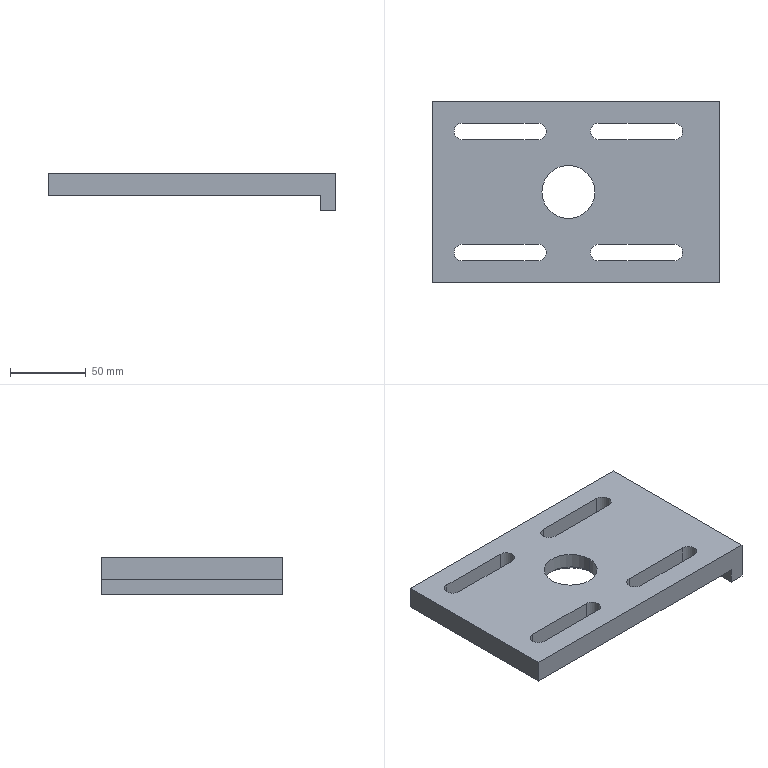Part | STEP file | Chain tension plate_default<machined> | 1 solid | 32 faces | box 190 x 120 x 25 mm | volume 299042 mm3 | plane 16 | cylinder 14 | cone 2 | commonest cylinder face diameters 11 x12 35 x2